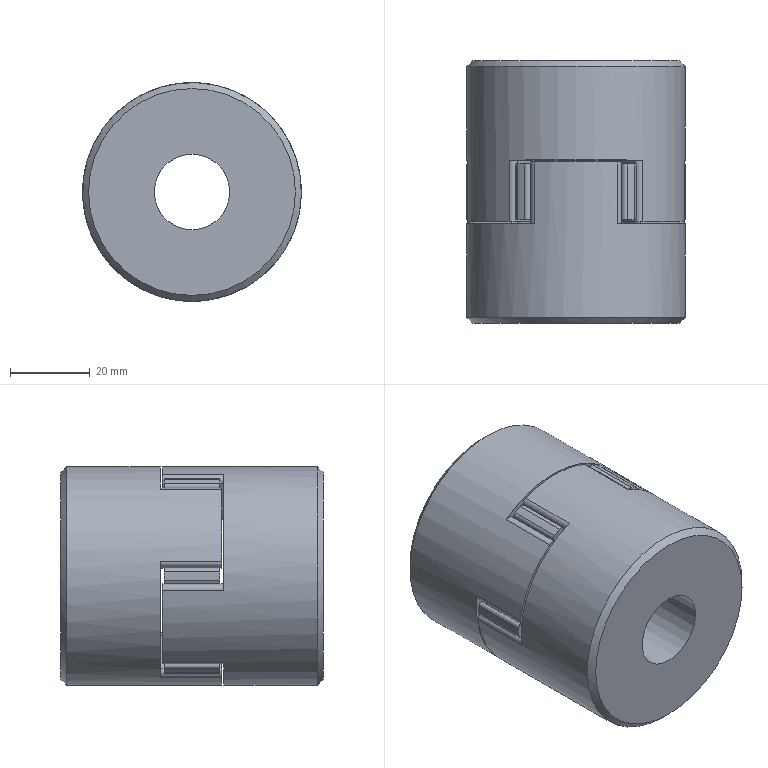Part | STEP file | YBQDJ-YB-17 | 1 solid | 145 faces | box 55 x 66 x 55 mm | volume 122440 mm3 | cylinder 83 | plane 60 | cone 2 | commonest cylinder face diameters 2 x24 3 x24 30 x24 55 x8 28 x2 19 x1